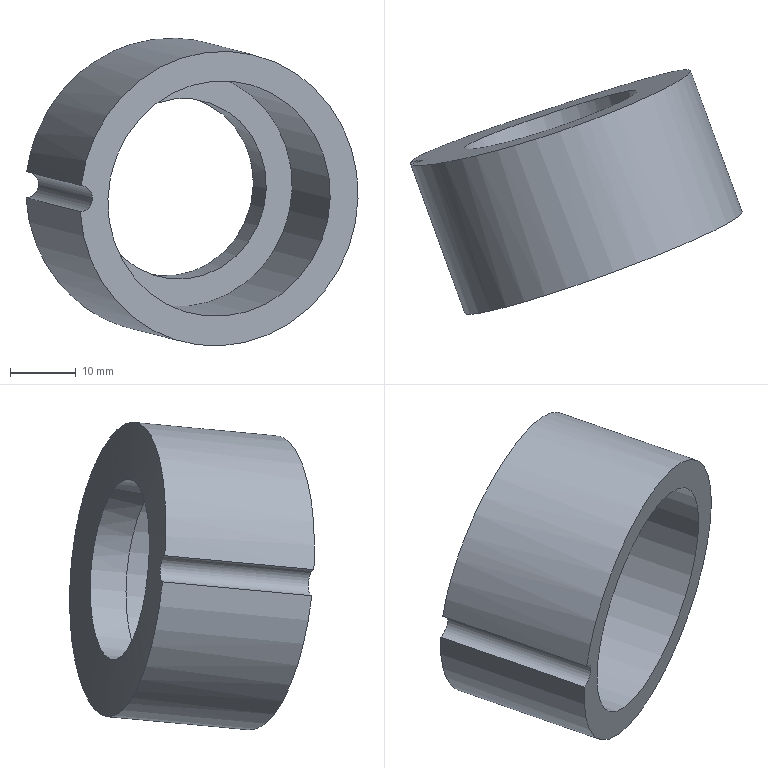Part | NX | features solid 2 | 1 solid | 7 faces | box 50.536 x 37.273 x 46.836 mm | volume 15739 mm3 | cylinder 4 | plane 2 | spline 1 | commonest cylinder face diameters 4 x1 27.62 x1 36 x1 45 x1
STEP:
#1=CARTESIAN_POINT('',(661.013,46.797,-29.339));
#2=VERTEX_POINT('',#1);
#3=CARTESIAN_POINT('',(677.928,52.954,-29.339));
#4=DIRECTION('',(-0.3407,0.9361,0.08716));
#5=DIRECTION('',(-0.9397,-0.342,0.));
#6=AXIS2_PLACEMENT_3D('',#3,#4,#5);
#7=CIRCLE('',#6,18.);
#8=EDGE_CURVE('',#2,#2,#7,.T.);
#9=ORIENTED_EDGE('',*,*,#8,.F.);
#10=EDGE_LOOP('',(#9));
#11=FACE_BOUND('',#10,.T.);
#12=CARTESIAN_POINT('',(664.951,48.23,-29.339));
#13=VERTEX_POINT('',#12);
#14=CARTESIAN_POINT('',(677.928,52.954,-29.339));
#15=DIRECTION('',(-0.3407,0.9361,0.08716));
#16=DIRECTION('',(-0.9397,-0.342,0.));
#17=AXIS2_PLACEMENT_3D('',#14,#15,#16);
#18=CIRCLE('',#17,13.81);
#19=EDGE_CURVE('',#13,#13,#18,.F.);
#20=ORIENTED_EDGE('',*,*,#19,.F.);
#21=EDGE_LOOP('',(#20));
#22=FACE_BOUND('',#21,.T.);
#23=CARTESIAN_POINT('',(677.928,52.954,-29.339));
#24=DIRECTION('',(0.3407,-0.9361,-0.08716));
#25=DIRECTION('',(-0.9397,-0.342,0.));
#26=AXIS2_PLACEMENT_3D('',#23,#24,#25);
#27=PLANE('',#26);
#28=ADVANCED_FACE('',(#11,#22),#27,.T.);
#29=CARTESIAN_POINT('',(654.338,52.242,-30.698));
#30=VERTEX_POINT('',#29);
#31=CARTESIAN_POINT('',(662.601,29.538,-32.811));
#32=VERTEX_POINT('',#31);
#33=CARTESIAN_POINT('',(658.415,41.04,-31.741));
#34=DIRECTION('',(0.3407,-0.9361,-0.08716));
#35=VECTOR('',#34,1000.);
#36=LINE('',#33,#35);
#37=EDGE_CURVE('',#30,#32,#36,.T.);
#38=ORIENTED_EDGE('',*,*,#37,.F.);
#39=CARTESIAN_POINT('',(654.46,51.905,-26.718));
#40=VERTEX_POINT('',#39);
#41=CARTESIAN_POINT('',(654.338,52.242,-30.698));
#42=CARTESIAN_POINT('',(654.496,52.548,-33.535));
#43=CARTESIAN_POINT('',(655.884,53.444,-39.131));
#44=CARTESIAN_POINT('',(660.851,55.473,-46.029));
#45=CARTESIAN_POINT('',(667.957,57.987,-50.456));
#46=CARTESIAN_POINT('',(676.16,60.715,-51.767));
#47=CARTESIAN_POINT('',(684.272,63.306,-49.763));
#48=CARTESIAN_POINT('',(691.133,65.354,-44.721));
#49=CARTESIAN_POINT('',(695.771,66.476,-37.387));
#50=CARTESIAN_POINT('',(697.559,66.42,-28.827));
#51=CARTESIAN_POINT('',(696.26,65.149,-20.276));
#52=CARTESIAN_POINT('',(692.055,62.87,-12.96));
#53=CARTESIAN_POINT('',(685.517,59.99,-7.921));
#54=CARTESIAN_POINT('',(677.55,57.015,-5.876));
#55=CARTESIAN_POINT('',(669.284,54.43,-7.12));
#56=CARTESIAN_POINT('',(659.439,51.975,-12.916));
#57=CARTESIAN_POINT('',(655.129,51.559,-21.019));
#58=CARTESIAN_POINT('',(654.46,51.905,-26.718));
#59=B_SPLINE_CURVE_WITH_KNOTS('',3,(#41,#42,#43,#44,#45,#46,#47,#48,#49,#50,#51,#52,#53,#54,#55,#56,#57,#58),.UNSPECIFIED.,.F.,.F.,(4,1,1,1,1,1,1,1,1,1,1,1,1,1,1,4),(0.001985,0.01053,0.01908,0.02763,0.03618,0.04472,0.05327,0.06182,0.07037,0.07892,0.08746,0.09601,0.1046,0.1131,0.1217,0.1388),.UNSPECIFIED.);
#60=EDGE_CURVE('',#30,#40,#59,.T.);
#61=ORIENTED_EDGE('',*,*,#60,.T.);
#62=CARTESIAN_POINT('',(662.72,29.211,-28.831));
#63=VERTEX_POINT('',#62);
#64=CARTESIAN_POINT('',(658.534,40.712,-27.76));
#65=DIRECTION('',(0.3407,-0.9361,-0.08716));
#66=VECTOR('',#65,1000.);
#67=LINE('',#64,#66);
#68=EDGE_CURVE('',#63,#40,#67,.F.);
#69=ORIENTED_EDGE('',*,*,#68,.F.);
#70=CARTESIAN_POINT('',(683.72,37.04,-30.821));
#71=DIRECTION('',(-0.3407,0.9361,0.08716));
#72=DIRECTION('',(-0.9397,-0.342,0.));
#73=AXIS2_PLACEMENT_3D('',#70,#71,#72);
#74=CIRCLE('',#73,22.5);
#75=EDGE_CURVE('',#63,#32,#74,.T.);
#76=ORIENTED_EDGE('',*,*,#75,.T.);
#77=EDGE_LOOP('',(#38,#61,#69,#76));
#78=FACE_BOUND('',#77,.T.);
#79=CARTESIAN_POINT('',(675.202,60.443,-28.642));
#80=DIRECTION('',(0.3407,-0.9361,-0.08716));
#81=DIRECTION('',(-0.9397,-0.342,0.));
#82=AXIS2_PLACEMENT_3D('',#79,#80,#81);
#83=CYLINDRICAL_SURFACE('',#82,22.5);
#84=ADVANCED_FACE('',(#78),#83,.T.);
#85=CARTESIAN_POINT('',(662.577,29.344,-30.821));
#86=DIRECTION('',(-0.3407,0.9361,0.08716));
#87=DIRECTION('',(-0.9397,-0.342,0.));
#88=AXIS2_PLACEMENT_3D('',#85,#86,#87);
#89=CIRCLE('',#88,2.);
#90=EDGE_CURVE('',#63,#32,#89,.T.);
#91=ORIENTED_EDGE('',*,*,#90,.T.);
#92=ORIENTED_EDGE('',*,*,#75,.F.);
#93=EDGE_LOOP('',(#91,#92));
#94=FACE_BOUND('',#93,.T.);
#95=CARTESIAN_POINT('',(666.806,30.883,-30.821));
#96=VERTEX_POINT('',#95);
#97=CARTESIAN_POINT('',(683.72,37.04,-30.821));
#98=DIRECTION('',(-0.3407,0.9361,0.08716));
#99=DIRECTION('',(-0.9397,-0.342,0.));
#100=AXIS2_PLACEMENT_3D('',#97,#98,#99);
#101=CIRCLE('',#100,18.);
#102=EDGE_CURVE('',#96,#96,#101,.T.);
#103=ORIENTED_EDGE('',*,*,#102,.T.);
#104=EDGE_LOOP('',(#103));
#105=FACE_BOUND('',#104,.T.);
#106=CARTESIAN_POINT('',(683.72,37.04,-30.821));
#107=DIRECTION('',(0.3407,-0.9361,-0.08716));
#108=DIRECTION('',(-0.9397,-0.342,0.));
#109=AXIS2_PLACEMENT_3D('',#106,#107,#108);
#110=PLANE('',#109);
#111=ADVANCED_FACE('',(#94,#105),#110,.T.);
#112=ORIENTED_EDGE('',*,*,#8,.T.);
#113=EDGE_LOOP('',(#112));
#114=FACE_BOUND('',#113,.T.);
#115=ORIENTED_EDGE('',*,*,#102,.F.);
#116=EDGE_LOOP('',(#115));
#117=FACE_BOUND('',#116,.T.);
#118=CARTESIAN_POINT('',(677.928,52.954,-29.339));
#119=DIRECTION('',(0.3407,-0.9361,-0.08716));
#120=DIRECTION('',(-0.9397,-0.342,0.));
#121=AXIS2_PLACEMENT_3D('',#118,#119,#120);
#122=CYLINDRICAL_SURFACE('',#121,18.);
#123=ADVANCED_FACE('',(#114,#117),#122,.F.);
#124=CARTESIAN_POINT('',(688.92,63.13,-28.832));
#125=VERTEX_POINT('',#124);
#126=CARTESIAN_POINT('',(686.422,61.227,-18.035));
#127=CARTESIAN_POINT('',(690.324,63.655,-28.833));
#128=CARTESIAN_POINT('',(685.804,62.935,-39.622));
#129=CARTESIAN_POINT('',(675.457,59.756,-44.066));
#130=CARTESIAN_POINT('',(665.249,56.168,-39.567));
#131=CARTESIAN_POINT('',(661.255,54.017,-28.756));
#132=CARTESIAN_POINT('',(665.885,54.373,-18.014));
#133=CARTESIAN_POINT('',(676.331,57.276,-13.574));
#134=CARTESIAN_POINT('',(686.422,61.227,-18.035));
#135=CARTESIAN_POINT('',(690.324,63.655,-28.833));
#136=CARTESIAN_POINT('',(685.804,62.935,-39.622));
#137=B_SPLINE_CURVE_WITH_KNOTS('',3,(#126,#127,#128,#129,#130,#131,#132,#133,#134,#135,#136),.UNSPECIFIED.,.T.,.F.,(1,1,1,1,1,1,1,1,1,1,1,1,1,1,1),(-0.03239,-0.02159,-0.0108,0.,0.0108,0.02159,0.03239,0.04318,0.05398,0.06478,0.07557,0.08637,0.09716,0.108,0.1188),.UNSPECIFIED.);
#138=EDGE_CURVE('',#125,#125,#137,.T.);
#139=ORIENTED_EDGE('',*,*,#138,.T.);
#140=EDGE_LOOP('',(#139));
#141=FACE_BOUND('',#140,.T.);
#142=ORIENTED_EDGE('',*,*,#19,.T.);
#143=EDGE_LOOP('',(#142));
#144=FACE_BOUND('',#143,.T.);
#145=CARTESIAN_POINT('',(692.238,13.637,-33.));
#146=DIRECTION('',(-0.3407,0.9361,0.08716));
#147=DIRECTION('',(0.9397,0.342,0.));
#148=AXIS2_PLACEMENT_3D('',#145,#146,#147);
#149=CYLINDRICAL_SURFACE('',#148,13.81);
#150=ADVANCED_FACE('',(#141,#144),#149,.F.);
#151=ORIENTED_EDGE('',*,*,#60,.F.);
#152=CARTESIAN_POINT('',(654.338,52.242,-30.698));
#153=CARTESIAN_POINT('',(654.83,52.374,-30.679));
#154=CARTESIAN_POINT('',(655.805,52.601,-30.237));
#155=CARTESIAN_POINT('',(656.445,52.639,-28.721));
#156=CARTESIAN_POINT('',(655.897,52.345,-27.199));
#157=CARTESIAN_POINT('',(654.951,52.042,-26.744));
#158=CARTESIAN_POINT('',(654.46,51.905,-26.718));
#159=B_SPLINE_CURVE_WITH_KNOTS('',3,(#152,#153,#154,#155,#156,#157,#158),.UNSPECIFIED.,.F.,.F.,(4,1,1,1,4),(0.003222,0.004743,0.006265,0.007786,0.009308),.UNSPECIFIED.);
#160=EDGE_CURVE('',#30,#40,#159,.T.);
#161=ORIENTED_EDGE('',*,*,#160,.T.);
#162=EDGE_LOOP('',(#151,#161));
#163=FACE_BOUND('',#162,.T.);
#164=ORIENTED_EDGE('',*,*,#138,.F.);
#165=EDGE_LOOP('',(#164));
#166=FACE_BOUND('',#165,.T.);
#167=CARTESIAN_POINT('',(653.269,49.795,-7.487));
#168=CARTESIAN_POINT('',(654.851,54.45,-52.968));
#169=CARTESIAN_POINT('',(667.966,53.707,-6.575));
#170=CARTESIAN_POINT('',(669.547,58.362,-52.056));
#171=CARTESIAN_POINT('',(682.425,58.41,-5.591));
#172=CARTESIAN_POINT('',(684.007,63.065,-51.072));
#173=CARTESIAN_POINT('',(696.604,63.89,-4.537));
#174=CARTESIAN_POINT('',(698.186,68.545,-50.018));
#175=(BOUNDED_SURFACE()B_SPLINE_SURFACE(3,1,((#167,#168),(#169,#170),(#171,#172),(#173,#174)),.SURF_OF_LINEAR_EXTRUSION.,.F.,.F.,.F.)B_SPLINE_SURFACE_WITH_KNOTS((4,4),(2,2),(0.3878,0.59),(0.3178,0.6831),.PIECEWISE_BEZIER_KNOTS.)GEOMETRIC_REPRESENTATION_ITEM()RATIONAL_B_SPLINE_SURFACE(((0.9969,0.9969),(0.9958,0.9958),(0.9957,0.9957),(0.9966,0.9966)))REPRESENTATION_ITEM('')SURFACE());
#176=ADVANCED_FACE('',(#163,#166),#175,.T.);
#177=ORIENTED_EDGE('',*,*,#37,.T.);
#178=ORIENTED_EDGE('',*,*,#90,.F.);
#179=ORIENTED_EDGE('',*,*,#68,.T.);
#180=ORIENTED_EDGE('',*,*,#160,.F.);
#181=EDGE_LOOP('',(#177,#178,#179,#180));
#182=FACE_BOUND('',#181,.T.);
#183=CARTESIAN_POINT('',(654.059,52.747,-28.642));
#184=DIRECTION('',(0.3407,-0.9361,-0.08716));
#185=DIRECTION('',(-0.9397,-0.342,0.));
#186=AXIS2_PLACEMENT_3D('',#183,#184,#185);
#187=CYLINDRICAL_SURFACE('',#186,2.);
#188=ADVANCED_FACE('',(#182),#187,.F.);
#189=CLOSED_SHELL('',(#28,#84,#111,#123,#150,#176,#188));
#190=MANIFOLD_SOLID_BREP('',#189);
#191=(LENGTH_UNIT()NAMED_UNIT(*)SI_UNIT(.MILLI.,.METRE.));
#192=UNCERTAINTY_MEASURE_WITH_UNIT(LENGTH_MEASURE(0.0508),#191,'','');
#193=(NAMED_UNIT(*)PLANE_ANGLE_UNIT()SI_UNIT($,.RADIAN.));
#194=(NAMED_UNIT(*)SI_UNIT($,.STERADIAN.)SOLID_ANGLE_UNIT());
#195=(GEOMETRIC_REPRESENTATION_CONTEXT(3)GLOBAL_UNCERTAINTY_ASSIGNED_CONTEXT((#192))GLOBAL_UNIT_ASSIGNED_CONTEXT((#191,#193,#194))REPRESENTATION_CONTEXT('',''));
#196=ADVANCED_BREP_SHAPE_REPRESENTATION('',(#190),#195);